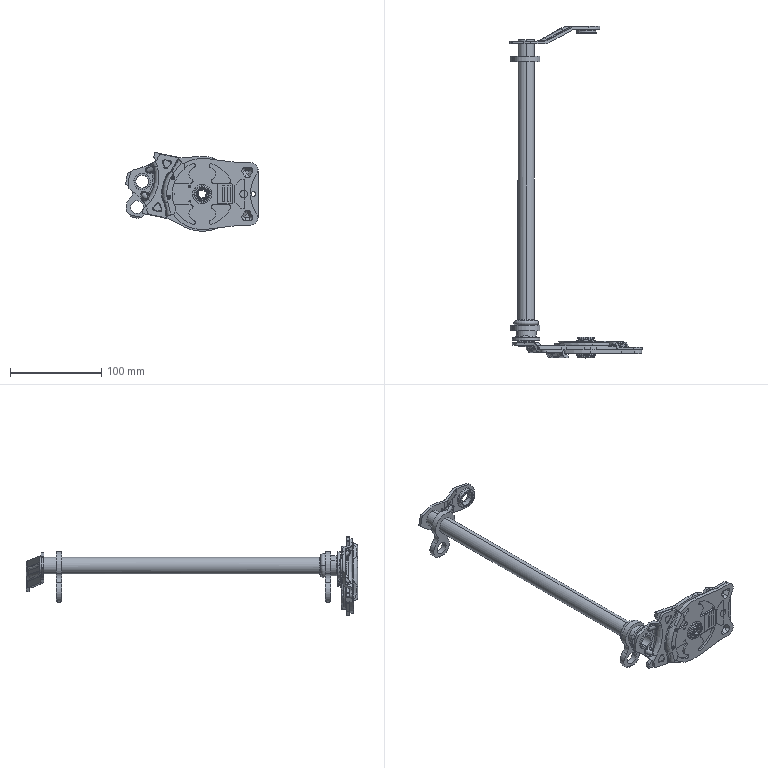Part | NX | features BREP 21 | 23 solids | 2428 faces | box 145.049 x 363 x 86.299 mm | volume 153863 mm3 | cylinder 916 | plane 657 | spline 436 | torus 219 | cone 168 | sphere 32 | commonest cylinder face diameters 0.3 x169 0.6 x144 1 x58 4 x40 2 x38 3 x32